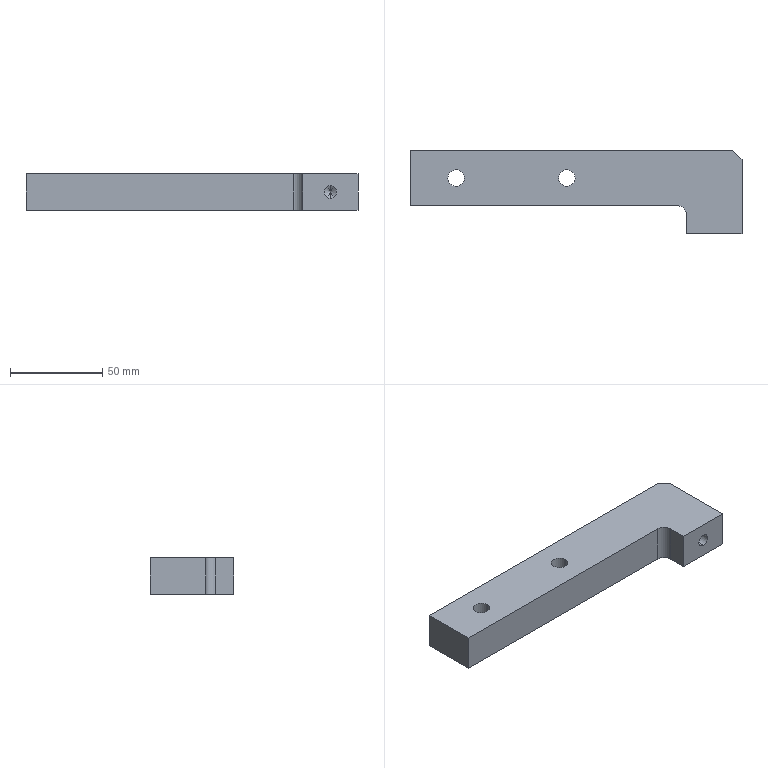Part | SolidWorks | features HoleWzd 2, Chamfer 1, Extrusion 1, Fillet 1, ICE 1 | 1 solid | 24 faces | box 180 x 45 x 20 mm | volume 111535 mm3 | cylinder 11 | plane 11 | cone 2 | commonest cylinder face diameters 9 x4 15 x4 6.8 x2 10 x1
STEP:
#1=CARTESIAN_POINT('',(2.5,0.,9.));
#2=VERTEX_POINT('',#1);
#3=CARTESIAN_POINT('',(-12.5,0.,9.));
#4=VERTEX_POINT('',#3);
#5=CARTESIAN_POINT('',(-5.,0.,9.));
#6=DIRECTION('',(0.,0.,-1.));
#7=DIRECTION('',(-1.,0.,0.));
#8=AXIS2_PLACEMENT_3D('',#5,#6,#7);
#9=CIRCLE('',#8,7.5);
#10=EDGE_CURVE('',#2,#4,#9,.T.);
#11=ORIENTED_EDGE('',*,*,#10,.F.);
#12=CARTESIAN_POINT('',(2.5,0.,0.));
#13=VERTEX_POINT('',#12);
#14=CARTESIAN_POINT('',(2.5,0.,0.));
#15=DIRECTION('',(0.,0.,-1.));
#16=VECTOR('',#15,1000.);
#17=LINE('',#14,#16);
#18=EDGE_CURVE('',#2,#13,#17,.T.);
#19=ORIENTED_EDGE('',*,*,#18,.T.);
#20=CARTESIAN_POINT('',(-12.5,0.,0.));
#21=VERTEX_POINT('',#20);
#22=CARTESIAN_POINT('',(-5.,0.,0.));
#23=DIRECTION('',(0.,0.,-1.));
#24=DIRECTION('',(-1.,0.,0.));
#25=AXIS2_PLACEMENT_3D('',#22,#23,#24);
#26=CIRCLE('',#25,7.5);
#27=EDGE_CURVE('',#13,#21,#26,.T.);
#28=ORIENTED_EDGE('',*,*,#27,.T.);
#29=CARTESIAN_POINT('',(-12.5,0.,0.));
#30=DIRECTION('',(0.,0.,-1.));
#31=VECTOR('',#30,1000.);
#32=LINE('',#29,#31);
#33=EDGE_CURVE('',#4,#21,#32,.T.);
#34=ORIENTED_EDGE('',*,*,#33,.F.);
#35=EDGE_LOOP('',(#11,#19,#28,#34));
#36=FACE_OUTER_BOUND('',#35,.T.);
#37=CARTESIAN_POINT('',(-5.,0.,0.));
#38=DIRECTION('',(0.,0.,-1.));
#39=DIRECTION('',(-1.,0.,0.));
#40=AXIS2_PLACEMENT_3D('',#37,#38,#39);
#41=CYLINDRICAL_SURFACE('',#40,7.5);
#42=ADVANCED_FACE('',(#36),#41,.F.);
#43=CARTESIAN_POINT('',(-9.5,0.,20.));
#44=VERTEX_POINT('',#43);
#45=CARTESIAN_POINT('',(-0.5,0.,20.));
#46=VERTEX_POINT('',#45);
#47=CARTESIAN_POINT('',(-5.,0.,20.));
#48=DIRECTION('',(0.,0.,1.));
#49=DIRECTION('',(1.,0.,0.));
#50=AXIS2_PLACEMENT_3D('',#47,#48,#49);
#51=CIRCLE('',#50,4.5);
#52=EDGE_CURVE('',#44,#46,#51,.T.);
#53=ORIENTED_EDGE('',*,*,#52,.T.);
#54=CARTESIAN_POINT('',(-0.5,0.,9.));
#55=VERTEX_POINT('',#54);
#56=CARTESIAN_POINT('',(-0.5,0.,0.));
#57=DIRECTION('',(0.,0.,-1.));
#58=VECTOR('',#57,1000.);
#59=LINE('',#56,#58);
#60=EDGE_CURVE('',#46,#55,#59,.T.);
#61=ORIENTED_EDGE('',*,*,#60,.T.);
#62=CARTESIAN_POINT('',(-9.5,0.,9.));
#63=VERTEX_POINT('',#62);
#64=CARTESIAN_POINT('',(-5.,0.,9.));
#65=DIRECTION('',(0.,0.,-1.));
#66=DIRECTION('',(-1.,0.,0.));
#67=AXIS2_PLACEMENT_3D('',#64,#65,#66);
#68=CIRCLE('',#67,4.5);
#69=EDGE_CURVE('',#55,#63,#68,.T.);
#70=ORIENTED_EDGE('',*,*,#69,.T.);
#71=CARTESIAN_POINT('',(-9.5,0.,0.));
#72=DIRECTION('',(0.,0.,-1.));
#73=VECTOR('',#72,1000.);
#74=LINE('',#71,#73);
#75=EDGE_CURVE('',#44,#63,#74,.T.);
#76=ORIENTED_EDGE('',*,*,#75,.F.);
#77=EDGE_LOOP('',(#53,#61,#70,#76));
#78=FACE_OUTER_BOUND('',#77,.T.);
#79=CARTESIAN_POINT('',(-5.,0.,0.));
#80=DIRECTION('',(0.,0.,-1.));
#81=DIRECTION('',(-1.,0.,0.));
#82=AXIS2_PLACEMENT_3D('',#79,#80,#81);
#83=CYLINDRICAL_SURFACE('',#82,4.5);
#84=ADVANCED_FACE('',(#78),#83,.F.);
#85=CARTESIAN_POINT('',(-57.5,0.,9.));
#86=VERTEX_POINT('',#85);
#87=CARTESIAN_POINT('',(-72.5,0.,9.));
#88=VERTEX_POINT('',#87);
#89=CARTESIAN_POINT('',(-65.,0.,9.));
#90=DIRECTION('',(0.,0.,-1.));
#91=DIRECTION('',(-1.,0.,0.));
#92=AXIS2_PLACEMENT_3D('',#89,#90,#91);
#93=CIRCLE('',#92,7.5);
#94=EDGE_CURVE('',#86,#88,#93,.T.);
#95=ORIENTED_EDGE('',*,*,#94,.F.);
#96=CARTESIAN_POINT('',(-57.5,0.,0.));
#97=VERTEX_POINT('',#96);
#98=CARTESIAN_POINT('',(-57.5,0.,0.));
#99=DIRECTION('',(0.,0.,-1.));
#100=VECTOR('',#99,1000.);
#101=LINE('',#98,#100);
#102=EDGE_CURVE('',#86,#97,#101,.T.);
#103=ORIENTED_EDGE('',*,*,#102,.T.);
#104=CARTESIAN_POINT('',(-72.5,0.,0.));
#105=VERTEX_POINT('',#104);
#106=CARTESIAN_POINT('',(-65.,0.,0.));
#107=DIRECTION('',(0.,0.,-1.));
#108=DIRECTION('',(-1.,0.,0.));
#109=AXIS2_PLACEMENT_3D('',#106,#107,#108);
#110=CIRCLE('',#109,7.5);
#111=EDGE_CURVE('',#97,#105,#110,.T.);
#112=ORIENTED_EDGE('',*,*,#111,.T.);
#113=CARTESIAN_POINT('',(-72.5,0.,0.));
#114=DIRECTION('',(0.,0.,-1.));
#115=VECTOR('',#114,1000.);
#116=LINE('',#113,#115);
#117=EDGE_CURVE('',#88,#105,#116,.T.);
#118=ORIENTED_EDGE('',*,*,#117,.F.);
#119=EDGE_LOOP('',(#95,#103,#112,#118));
#120=FACE_OUTER_BOUND('',#119,.T.);
#121=CARTESIAN_POINT('',(-65.,0.,0.));
#122=DIRECTION('',(0.,0.,-1.));
#123=DIRECTION('',(-1.,0.,0.));
#124=AXIS2_PLACEMENT_3D('',#121,#122,#123);
#125=CYLINDRICAL_SURFACE('',#124,7.5);
#126=ADVANCED_FACE('',(#120),#125,.F.);
#127=CARTESIAN_POINT('',(-69.5,0.,20.));
#128=VERTEX_POINT('',#127);
#129=CARTESIAN_POINT('',(-60.5,0.,20.));
#130=VERTEX_POINT('',#129);
#131=CARTESIAN_POINT('',(-65.,0.,20.));
#132=DIRECTION('',(0.,0.,1.));
#133=DIRECTION('',(1.,0.,0.));
#134=AXIS2_PLACEMENT_3D('',#131,#132,#133);
#135=CIRCLE('',#134,4.5);
#136=EDGE_CURVE('',#128,#130,#135,.T.);
#137=ORIENTED_EDGE('',*,*,#136,.T.);
#138=CARTESIAN_POINT('',(-60.5,0.,9.));
#139=VERTEX_POINT('',#138);
#140=CARTESIAN_POINT('',(-60.5,0.,0.));
#141=DIRECTION('',(0.,0.,-1.));
#142=VECTOR('',#141,1000.);
#143=LINE('',#140,#142);
#144=EDGE_CURVE('',#130,#139,#143,.T.);
#145=ORIENTED_EDGE('',*,*,#144,.T.);
#146=CARTESIAN_POINT('',(-69.5,0.,9.));
#147=VERTEX_POINT('',#146);
#148=CARTESIAN_POINT('',(-65.,0.,9.));
#149=DIRECTION('',(0.,0.,-1.));
#150=DIRECTION('',(-1.,0.,0.));
#151=AXIS2_PLACEMENT_3D('',#148,#149,#150);
#152=CIRCLE('',#151,4.5);
#153=EDGE_CURVE('',#139,#147,#152,.T.);
#154=ORIENTED_EDGE('',*,*,#153,.T.);
#155=CARTESIAN_POINT('',(-69.5,0.,0.));
#156=DIRECTION('',(0.,0.,-1.));
#157=VECTOR('',#156,1000.);
#158=LINE('',#155,#157);
#159=EDGE_CURVE('',#128,#147,#158,.T.);
#160=ORIENTED_EDGE('',*,*,#159,.F.);
#161=EDGE_LOOP('',(#137,#145,#154,#160));
#162=FACE_OUTER_BOUND('',#161,.T.);
#163=CARTESIAN_POINT('',(-65.,0.,0.));
#164=DIRECTION('',(0.,0.,-1.));
#165=DIRECTION('',(-1.,0.,0.));
#166=AXIS2_PLACEMENT_3D('',#163,#164,#165);
#167=CYLINDRICAL_SURFACE('',#166,4.5);
#168=ADVANCED_FACE('',(#162),#167,.F.);
#169=CARTESIAN_POINT('',(75.,-10.25,13.4));
#170=VERTEX_POINT('',#169);
#171=CARTESIAN_POINT('',(75.,-10.25,6.6));
#172=VERTEX_POINT('',#171);
#173=CARTESIAN_POINT('',(75.,-10.25,10.));
#174=DIRECTION('',(0.,-1.,0.));
#175=DIRECTION('',(0.,0.,-1.));
#176=AXIS2_PLACEMENT_3D('',#173,#174,#175);
#177=CIRCLE('',#176,3.4);
#178=EDGE_CURVE('',#170,#172,#177,.T.);
#179=ORIENTED_EDGE('',*,*,#178,.F.);
#180=CARTESIAN_POINT('',(75.,-30.,13.4));
#181=VERTEX_POINT('',#180);
#182=CARTESIAN_POINT('',(75.,-30.,13.4));
#183=DIRECTION('',(0.,-1.,0.));
#184=VECTOR('',#183,1000.);
#185=LINE('',#182,#184);
#186=EDGE_CURVE('',#170,#181,#185,.T.);
#187=ORIENTED_EDGE('',*,*,#186,.T.);
#188=CARTESIAN_POINT('',(75.,-30.,6.6));
#189=VERTEX_POINT('',#188);
#190=CARTESIAN_POINT('',(75.,-30.,10.));
#191=DIRECTION('',(0.,-1.,0.));
#192=DIRECTION('',(0.,0.,-1.));
#193=AXIS2_PLACEMENT_3D('',#190,#191,#192);
#194=CIRCLE('',#193,3.4);
#195=EDGE_CURVE('',#181,#189,#194,.T.);
#196=ORIENTED_EDGE('',*,*,#195,.T.);
#197=CARTESIAN_POINT('',(75.,-30.,6.6));
#198=DIRECTION('',(0.,-1.,0.));
#199=VECTOR('',#198,1000.);
#200=LINE('',#197,#199);
#201=EDGE_CURVE('',#172,#189,#200,.T.);
#202=ORIENTED_EDGE('',*,*,#201,.F.);
#203=EDGE_LOOP('',(#179,#187,#196,#202));
#204=FACE_OUTER_BOUND('',#203,.T.);
#205=CARTESIAN_POINT('',(75.,-30.,10.));
#206=DIRECTION('',(0.,-1.,0.));
#207=DIRECTION('',(0.,0.,-1.));
#208=AXIS2_PLACEMENT_3D('',#205,#206,#207);
#209=CYLINDRICAL_SURFACE('',#208,3.4);
#210=ADVANCED_FACE('',(#204),#209,.F.);
#211=CARTESIAN_POINT('',(75.,-8.207,10.));
#212=VERTEX_POINT('',#211);
#213=CARTESIAN_POINT('',(75.,-10.25,6.6));
#214=DIRECTION('',(0.,-0.515,-0.8572));
#215=VECTOR('',#214,1000.);
#216=LINE('',#213,#215);
#217=EDGE_CURVE('',#212,#172,#216,.T.);
#218=ORIENTED_EDGE('',*,*,#217,.F.);
#219=CARTESIAN_POINT('',(75.,-10.25,13.4));
#220=DIRECTION('',(0.,-0.515,0.8572));
#221=VECTOR('',#220,1000.);
#222=LINE('',#219,#221);
#223=EDGE_CURVE('',#212,#170,#222,.T.);
#224=ORIENTED_EDGE('',*,*,#223,.T.);
#225=ORIENTED_EDGE('',*,*,#178,.T.);
#226=EDGE_LOOP('',(#218,#224,#225));
#227=FACE_OUTER_BOUND('',#226,.T.);
#228=CARTESIAN_POINT('',(75.,-10.25,10.));
#229=DIRECTION('',(0.,-1.,0.));
#230=DIRECTION('',(0.,0.,-1.));
#231=AXIS2_PLACEMENT_3D('',#228,#229,#230);
#232=CONICAL_SURFACE('',#231,3.4,1.03);
#233=ADVANCED_FACE('',(#227),#232,.F.);
#234=CARTESIAN_POINT('',(90.,-30.,0.));
#235=VERTEX_POINT('',#234);
#236=CARTESIAN_POINT('',(90.,10.,0.));
#237=VERTEX_POINT('',#236);
#238=CARTESIAN_POINT('',(90.,15.,0.));
#239=DIRECTION('',(0.,1.,0.));
#240=VECTOR('',#239,1000.);
#241=LINE('',#238,#240);
#242=EDGE_CURVE('',#235,#237,#241,.T.);
#243=ORIENTED_EDGE('',*,*,#242,.T.);
#244=CARTESIAN_POINT('',(90.,10.,20.));
#245=VERTEX_POINT('',#244);
#246=CARTESIAN_POINT('',(90.,10.,20.));
#247=DIRECTION('',(0.,0.,1.));
#248=VECTOR('',#247,1000.);
#249=LINE('',#246,#248);
#250=EDGE_CURVE('',#237,#245,#249,.T.);
#251=ORIENTED_EDGE('',*,*,#250,.T.);
#252=CARTESIAN_POINT('',(90.,-30.,20.));
#253=VERTEX_POINT('',#252);
#254=CARTESIAN_POINT('',(90.,15.,20.));
#255=DIRECTION('',(0.,1.,0.));
#256=VECTOR('',#255,1000.);
#257=LINE('',#254,#256);
#258=EDGE_CURVE('',#253,#245,#257,.T.);
#259=ORIENTED_EDGE('',*,*,#258,.F.);
#260=CARTESIAN_POINT('',(90.,-30.,-33.541));
#261=DIRECTION('',(0.,0.,1.));
#262=VECTOR('',#261,1000.);
#263=LINE('',#260,#262);
#264=EDGE_CURVE('',#235,#253,#263,.T.);
#265=ORIENTED_EDGE('',*,*,#264,.F.);
#266=EDGE_LOOP('',(#243,#251,#259,#265));
#267=FACE_OUTER_BOUND('',#266,.T.);
#268=CARTESIAN_POINT('',(90.,15.,20.));
#269=DIRECTION('',(-1.,0.,0.));
#270=DIRECTION('',(0.,0.,1.));
#271=AXIS2_PLACEMENT_3D('',#268,#269,#270);
#272=PLANE('',#271);
#273=ADVANCED_FACE('',(#267),#272,.F.);
#274=CARTESIAN_POINT('',(85.,15.,20.));
#275=VERTEX_POINT('',#274);
#276=CARTESIAN_POINT('',(-90.,15.,20.));
#277=VERTEX_POINT('',#276);
#278=CARTESIAN_POINT('',(-90.,15.,20.));
#279=DIRECTION('',(-1.,0.,0.));
#280=VECTOR('',#279,1000.);
#281=LINE('',#278,#280);
#282=EDGE_CURVE('',#275,#277,#281,.T.);
#283=ORIENTED_EDGE('',*,*,#282,.F.);
#284=CARTESIAN_POINT('',(85.,15.,0.));
#285=VERTEX_POINT('',#284);
#286=CARTESIAN_POINT('',(85.,15.,20.));
#287=DIRECTION('',(0.,0.,-1.));
#288=VECTOR('',#287,1000.);
#289=LINE('',#286,#288);
#290=EDGE_CURVE('',#275,#285,#289,.T.);
#291=ORIENTED_EDGE('',*,*,#290,.T.);
#292=CARTESIAN_POINT('',(-90.,15.,0.));
#293=VERTEX_POINT('',#292);
#294=CARTESIAN_POINT('',(-90.,15.,0.));
#295=DIRECTION('',(-1.,0.,0.));
#296=VECTOR('',#295,1000.);
#297=LINE('',#294,#296);
#298=EDGE_CURVE('',#285,#293,#297,.T.);
#299=ORIENTED_EDGE('',*,*,#298,.T.);
#300=CARTESIAN_POINT('',(-90.,15.,20.));
#301=DIRECTION('',(0.,0.,-1.));
#302=VECTOR('',#301,1000.);
#303=LINE('',#300,#302);
#304=EDGE_CURVE('',#277,#293,#303,.T.);
#305=ORIENTED_EDGE('',*,*,#304,.F.);
#306=EDGE_LOOP('',(#283,#291,#299,#305));
#307=FACE_OUTER_BOUND('',#306,.T.);
#308=CARTESIAN_POINT('',(-90.,15.,20.));
#309=DIRECTION('',(0.,-1.,0.));
#310=DIRECTION('',(0.,0.,-1.));
#311=AXIS2_PLACEMENT_3D('',#308,#309,#310);
#312=PLANE('',#311);
#313=ADVANCED_FACE('',(#307),#312,.F.);
#314=CARTESIAN_POINT('',(-90.,-15.,0.));
#315=VERTEX_POINT('',#314);
#316=CARTESIAN_POINT('',(-90.,15.,0.));
#317=DIRECTION('',(0.,-1.,0.));
#318=VECTOR('',#317,1000.);
#319=LINE('',#316,#318);
#320=EDGE_CURVE('',#293,#315,#319,.T.);
#321=ORIENTED_EDGE('',*,*,#320,.T.);
#322=CARTESIAN_POINT('',(-90.,-15.,20.));
#323=VERTEX_POINT('',#322);
#324=CARTESIAN_POINT('',(-90.,-15.,20.));
#325=DIRECTION('',(0.,0.,-1.));
#326=VECTOR('',#325,1000.);
#327=LINE('',#324,#326);
#328=EDGE_CURVE('',#323,#315,#327,.T.);
#329=ORIENTED_EDGE('',*,*,#328,.F.);
#330=CARTESIAN_POINT('',(-90.,15.,20.));
#331=DIRECTION('',(0.,-1.,0.));
#332=VECTOR('',#331,1000.);
#333=LINE('',#330,#332);
#334=EDGE_CURVE('',#277,#323,#333,.T.);
#335=ORIENTED_EDGE('',*,*,#334,.F.);
#336=ORIENTED_EDGE('',*,*,#304,.T.);
#337=EDGE_LOOP('',(#321,#329,#335,#336));
#338=FACE_OUTER_BOUND('',#337,.T.);
#339=CARTESIAN_POINT('',(-90.,15.,20.));
#340=DIRECTION('',(1.,0.,0.));
#341=DIRECTION('',(0.,0.,-1.));
#342=AXIS2_PLACEMENT_3D('',#339,#340,#341);
#343=PLANE('',#342);
#344=ADVANCED_FACE('',(#338),#343,.F.);
#345=CARTESIAN_POINT('',(55.,-15.,0.));
#346=VERTEX_POINT('',#345);
#347=CARTESIAN_POINT('',(-90.,-15.,0.));
#348=DIRECTION('',(1.,0.,0.));
#349=VECTOR('',#348,1000.);
#350=LINE('',#347,#349);
#351=EDGE_CURVE('',#315,#346,#350,.T.);
#352=ORIENTED_EDGE('',*,*,#351,.T.);
#353=CARTESIAN_POINT('',(55.,-15.,20.));
#354=VERTEX_POINT('',#353);
#355=CARTESIAN_POINT('',(55.,-15.,20.));
#356=DIRECTION('',(0.,0.,1.));
#357=VECTOR('',#356,1000.);
#358=LINE('',#355,#357);
#359=EDGE_CURVE('',#346,#354,#358,.T.);
#360=ORIENTED_EDGE('',*,*,#359,.T.);
#361=CARTESIAN_POINT('',(-90.,-15.,20.));
#362=DIRECTION('',(1.,0.,0.));
#363=VECTOR('',#362,1000.);
#364=LINE('',#361,#363);
#365=EDGE_CURVE('',#323,#354,#364,.T.);
#366=ORIENTED_EDGE('',*,*,#365,.F.);
#367=ORIENTED_EDGE('',*,*,#328,.T.);
#368=EDGE_LOOP('',(#352,#360,#366,#367));
#369=FACE_OUTER_BOUND('',#368,.T.);
#370=CARTESIAN_POINT('',(-90.,-15.,20.));
#371=DIRECTION('',(0.,1.,0.));
#372=DIRECTION('',(0.,0.,1.));
#373=AXIS2_PLACEMENT_3D('',#370,#371,#372);
#374=PLANE('',#373);
#375=ADVANCED_FACE('',(#369),#374,.F.);
#376=ORIENTED_EDGE('',*,*,#52,.F.);
#377=CARTESIAN_POINT('',(-5.,0.,20.));
#378=DIRECTION('',(0.,0.,1.));
#379=DIRECTION('',(1.,0.,0.));
#380=AXIS2_PLACEMENT_3D('',#377,#378,#379);
#381=CIRCLE('',#380,4.5);
#382=EDGE_CURVE('',#46,#44,#381,.T.);
#383=ORIENTED_EDGE('',*,*,#382,.F.);
#384=EDGE_LOOP('',(#376,#383));
#385=FACE_BOUND('',#384,.T.);
#386=ORIENTED_EDGE('',*,*,#136,.F.);
#387=CARTESIAN_POINT('',(-65.,0.,20.));
#388=DIRECTION('',(0.,0.,1.));
#389=DIRECTION('',(1.,0.,0.));
#390=AXIS2_PLACEMENT_3D('',#387,#388,#389);
#391=CIRCLE('',#390,4.5);
#392=EDGE_CURVE('',#130,#128,#391,.T.);
#393=ORIENTED_EDGE('',*,*,#392,.F.);
#394=EDGE_LOOP('',(#386,#393));
#395=FACE_BOUND('',#394,.T.);
#396=ORIENTED_EDGE('',*,*,#258,.T.);
#397=CARTESIAN_POINT('',(50.,50.,20.));
#398=DIRECTION('',(-0.7071,0.7071,0.));
#399=VECTOR('',#398,1000.);
#400=LINE('',#397,#399);
#401=EDGE_CURVE('',#245,#275,#400,.T.);
#402=ORIENTED_EDGE('',*,*,#401,.T.);
#403=ORIENTED_EDGE('',*,*,#282,.T.);
#404=ORIENTED_EDGE('',*,*,#334,.T.);
#405=ORIENTED_EDGE('',*,*,#365,.T.);
#406=CARTESIAN_POINT('',(60.,-20.,20.));
#407=VERTEX_POINT('',#406);
#408=CARTESIAN_POINT('',(55.,-20.,20.));
#409=DIRECTION('',(0.,0.,-1.));
#410=DIRECTION('',(1.,0.,0.));
#411=AXIS2_PLACEMENT_3D('',#408,#409,#410);
#412=CIRCLE('',#411,5.);
#413=EDGE_CURVE('',#354,#407,#412,.T.);
#414=ORIENTED_EDGE('',*,*,#413,.T.);
#415=CARTESIAN_POINT('',(60.,-30.,20.));
#416=VERTEX_POINT('',#415);
#417=CARTESIAN_POINT('',(60.,-30.,20.));
#418=DIRECTION('',(0.,1.,0.));
#419=VECTOR('',#418,1000.);
#420=LINE('',#417,#419);
#421=EDGE_CURVE('',#416,#407,#420,.T.);
#422=ORIENTED_EDGE('',*,*,#421,.F.);
#423=CARTESIAN_POINT('',(90.,-30.,20.));
#424=DIRECTION('',(-1.,0.,0.));
#425=VECTOR('',#424,1000.);
#426=LINE('',#423,#425);
#427=EDGE_CURVE('',#253,#416,#426,.T.);
#428=ORIENTED_EDGE('',*,*,#427,.F.);
#429=EDGE_LOOP('',(#396,#402,#403,#404,#405,#414,#422,#428));
#430=FACE_OUTER_BOUND('',#429,.T.);
#431=CARTESIAN_POINT('',(0.,0.,20.));
#432=DIRECTION('',(0.,0.,1.));
#433=DIRECTION('',(1.,0.,0.));
#434=AXIS2_PLACEMENT_3D('',#431,#432,#433);
#435=PLANE('',#434);
#436=ADVANCED_FACE('',(#385,#395,#430),#435,.T.);
#437=CARTESIAN_POINT('',(-5.,0.,0.));
#438=DIRECTION('',(0.,0.,-1.));
#439=DIRECTION('',(-1.,0.,0.));
#440=AXIS2_PLACEMENT_3D('',#437,#438,#439);
#441=CIRCLE('',#440,7.5);
#442=EDGE_CURVE('',#21,#13,#441,.T.);
#443=ORIENTED_EDGE('',*,*,#442,.F.);
#444=ORIENTED_EDGE('',*,*,#27,.F.);
#445=EDGE_LOOP('',(#443,#444));
#446=FACE_BOUND('',#445,.T.);
#447=CARTESIAN_POINT('',(-65.,0.,0.));
#448=DIRECTION('',(0.,0.,-1.));
#449=DIRECTION('',(-1.,0.,0.));
#450=AXIS2_PLACEMENT_3D('',#447,#448,#449);
#451=CIRCLE('',#450,7.5);
#452=EDGE_CURVE('',#105,#97,#451,.T.);
#453=ORIENTED_EDGE('',*,*,#452,.F.);
#454=ORIENTED_EDGE('',*,*,#111,.F.);
#455=EDGE_LOOP('',(#453,#454));
#456=FACE_BOUND('',#455,.T.);
#457=ORIENTED_EDGE('',*,*,#298,.F.);
#458=CARTESIAN_POINT('',(85.,15.,0.));
#459=DIRECTION('',(0.7071,-0.7071,0.));
#460=VECTOR('',#459,1000.);
#461=LINE('',#458,#460);
#462=EDGE_CURVE('',#285,#237,#461,.T.);
#463=ORIENTED_EDGE('',*,*,#462,.T.);
#464=ORIENTED_EDGE('',*,*,#242,.F.);
#465=CARTESIAN_POINT('',(60.,-30.,0.));
#466=VERTEX_POINT('',#465);
#467=CARTESIAN_POINT('',(90.,-30.,0.));
#468=DIRECTION('',(1.,0.,0.));
#469=VECTOR('',#468,1000.);
#470=LINE('',#467,#469);
#471=EDGE_CURVE('',#466,#235,#470,.T.);
#472=ORIENTED_EDGE('',*,*,#471,.F.);
#473=CARTESIAN_POINT('',(60.,-20.,0.));
#474=VERTEX_POINT('',#473);
#475=CARTESIAN_POINT('',(60.,-30.,0.));
#476=DIRECTION('',(0.,-1.,0.));
#477=VECTOR('',#476,1000.);
#478=LINE('',#475,#477);
#479=EDGE_CURVE('',#474,#466,#478,.T.);
#480=ORIENTED_EDGE('',*,*,#479,.F.);
#481=CARTESIAN_POINT('',(55.,-20.,0.));
#482=DIRECTION('',(0.,0.,1.));
#483=DIRECTION('',(1.,0.,0.));
#484=AXIS2_PLACEMENT_3D('',#481,#482,#483);
#485=CIRCLE('',#484,5.);
#486=EDGE_CURVE('',#474,#346,#485,.T.);
#487=ORIENTED_EDGE('',*,*,#486,.T.);
#488=ORIENTED_EDGE('',*,*,#351,.F.);
#489=ORIENTED_EDGE('',*,*,#320,.F.);
#490=EDGE_LOOP('',(#457,#463,#464,#472,#480,#487,#488,#489));
#491=FACE_OUTER_BOUND('',#490,.T.);
#492=CARTESIAN_POINT('',(0.,0.,0.));
#493=DIRECTION('',(0.,0.,1.));
#494=DIRECTION('',(1.,0.,0.));
#495=AXIS2_PLACEMENT_3D('',#492,#493,#494);
#496=PLANE('',#495);
#497=ADVANCED_FACE('',(#446,#456,#491),#496,.F.);
#498=ORIENTED_EDGE('',*,*,#421,.T.);
#499=CARTESIAN_POINT('',(60.,-20.,0.));
#500=DIRECTION('',(0.,0.,-1.));
#501=VECTOR('',#500,1000.);
#502=LINE('',#499,#501);
#503=EDGE_CURVE('',#407,#474,#502,.T.);
#504=ORIENTED_EDGE('',*,*,#503,.T.);
#505=ORIENTED_EDGE('',*,*,#479,.T.);
#506=CARTESIAN_POINT('',(60.,-30.,-33.541));
#507=DIRECTION('',(0.,0.,1.));
#508=VECTOR('',#507,1000.);
#509=LINE('',#506,#508);
#510=EDGE_CURVE('',#466,#416,#509,.T.);
#511=ORIENTED_EDGE('',*,*,#510,.T.);
#512=EDGE_LOOP('',(#498,#504,#505,#511));
#513=FACE_OUTER_BOUND('',#512,.T.);
#514=CARTESIAN_POINT('',(60.,-30.,-33.541));
#515=DIRECTION('',(1.,0.,0.));
#516=DIRECTION('',(0.,0.,-1.));
#517=AXIS2_PLACEMENT_3D('',#514,#515,#516);
#518=PLANE('',#517);
#519=ADVANCED_FACE('',(#513),#518,.F.);
#520=CARTESIAN_POINT('',(75.,-30.,10.));
#521=DIRECTION('',(0.,-1.,0.));
#522=DIRECTION('',(0.,0.,-1.));
#523=AXIS2_PLACEMENT_3D('',#520,#521,#522);
#524=CIRCLE('',#523,3.4);
#525=EDGE_CURVE('',#189,#181,#524,.T.);
#526=ORIENTED_EDGE('',*,*,#525,.F.);
#527=ORIENTED_EDGE('',*,*,#195,.F.);
#528=EDGE_LOOP('',(#526,#527));
#529=FACE_BOUND('',#528,.T.);
#530=ORIENTED_EDGE('',*,*,#510,.F.);
#531=ORIENTED_EDGE('',*,*,#471,.T.);
#532=ORIENTED_EDGE('',*,*,#264,.T.);
#533=ORIENTED_EDGE('',*,*,#427,.T.);
#534=EDGE_LOOP('',(#530,#531,#532,#533));
#535=FACE_OUTER_BOUND('',#534,.T.);
#536=CARTESIAN_POINT('',(90.,-30.,-33.541));
#537=DIRECTION('',(0.,1.,0.));
#538=DIRECTION('',(-1.,0.,0.));
#539=AXIS2_PLACEMENT_3D('',#536,#537,#538);
#540=PLANE('',#539);
#541=ADVANCED_FACE('',(#529,#535),#540,.F.);
#542=ORIENTED_EDGE('',*,*,#486,.F.);
#543=ORIENTED_EDGE('',*,*,#503,.F.);
#544=ORIENTED_EDGE('',*,*,#413,.F.);
#545=ORIENTED_EDGE('',*,*,#359,.F.);
#546=EDGE_LOOP('',(#542,#543,#544,#545));
#547=FACE_OUTER_BOUND('',#546,.T.);
#548=CARTESIAN_POINT('',(55.,-20.,20.));
#549=DIRECTION('',(0.,0.,-1.));
#550=DIRECTION('',(-1.,0.,0.));
#551=AXIS2_PLACEMENT_3D('',#548,#549,#550);
#552=CYLINDRICAL_SURFACE('',#551,5.);
#553=ADVANCED_FACE('',(#547),#552,.F.);
#554=ORIENTED_EDGE('',*,*,#401,.F.);
#555=ORIENTED_EDGE('',*,*,#250,.F.);
#556=ORIENTED_EDGE('',*,*,#462,.F.);
#557=ORIENTED_EDGE('',*,*,#290,.F.);
#558=EDGE_LOOP('',(#554,#555,#556,#557));
#559=FACE_OUTER_BOUND('',#558,.T.);
#560=CARTESIAN_POINT('',(85.,15.,20.));
#561=DIRECTION('',(-0.7071,-0.7071,0.));
#562=DIRECTION('',(0.,0.,-1.));
#563=AXIS2_PLACEMENT_3D('',#560,#561,#562);
#564=PLANE('',#563);
#565=ADVANCED_FACE('',(#559),#564,.F.);
#566=ORIENTED_EDGE('',*,*,#223,.F.);
#567=ORIENTED_EDGE('',*,*,#217,.T.);
#568=CARTESIAN_POINT('',(75.,-10.25,10.));
#569=DIRECTION('',(0.,-1.,0.));
#570=DIRECTION('',(0.,0.,-1.));
#571=AXIS2_PLACEMENT_3D('',#568,#569,#570);
#572=CIRCLE('',#571,3.4);
#573=EDGE_CURVE('',#172,#170,#572,.T.);
#574=ORIENTED_EDGE('',*,*,#573,.T.);
#575=EDGE_LOOP('',(#566,#567,#574));
#576=FACE_OUTER_BOUND('',#575,.T.);
#577=CARTESIAN_POINT('',(75.,-10.25,10.));
#578=DIRECTION('',(0.,-1.,0.));
#579=DIRECTION('',(0.,0.,-1.));
#580=AXIS2_PLACEMENT_3D('',#577,#578,#579);
#581=CONICAL_SURFACE('',#580,3.4,1.03);
#582=ADVANCED_FACE('',(#576),#581,.F.);
#583=ORIENTED_EDGE('',*,*,#186,.F.);
#584=ORIENTED_EDGE('',*,*,#573,.F.);
#585=ORIENTED_EDGE('',*,*,#201,.T.);
#586=ORIENTED_EDGE('',*,*,#525,.T.);
#587=EDGE_LOOP('',(#583,#584,#585,#586));
#588=FACE_OUTER_BOUND('',#587,.T.);
#589=CARTESIAN_POINT('',(75.,-30.,10.));
#590=DIRECTION('',(0.,-1.,0.));
#591=DIRECTION('',(0.,0.,-1.));
#592=AXIS2_PLACEMENT_3D('',#589,#590,#591);
#593=CYLINDRICAL_SURFACE('',#592,3.4);
#594=ADVANCED_FACE('',(#588),#593,.F.);
#595=ORIENTED_EDGE('',*,*,#144,.F.);
#596=ORIENTED_EDGE('',*,*,#392,.T.);
#597=ORIENTED_EDGE('',*,*,#159,.T.);
#598=CARTESIAN_POINT('',(-65.,0.,9.));
#599=DIRECTION('',(0.,0.,-1.));
#600=DIRECTION('',(-1.,0.,0.));
#601=AXIS2_PLACEMENT_3D('',#598,#599,#600);
#602=CIRCLE('',#601,4.5);
#603=EDGE_CURVE('',#147,#139,#602,.T.);
#604=ORIENTED_EDGE('',*,*,#603,.T.);
#605=EDGE_LOOP('',(#595,#596,#597,#604));
#606=FACE_OUTER_BOUND('',#605,.T.);
#607=CARTESIAN_POINT('',(-65.,0.,0.));
#608=DIRECTION('',(0.,0.,-1.));
#609=DIRECTION('',(-1.,0.,0.));
#610=AXIS2_PLACEMENT_3D('',#607,#608,#609);
#611=CYLINDRICAL_SURFACE('',#610,4.5);
#612=ADVANCED_FACE('',(#606),#611,.F.);
#613=ORIENTED_EDGE('',*,*,#603,.F.);
#614=ORIENTED_EDGE('',*,*,#153,.F.);
#615=EDGE_LOOP('',(#613,#614));
#616=FACE_BOUND('',#615,.T.);
#617=CARTESIAN_POINT('',(-65.,0.,9.));
#618=DIRECTION('',(0.,0.,-1.));
#619=DIRECTION('',(-1.,0.,0.));
#620=AXIS2_PLACEMENT_3D('',#617,#618,#619);
#621=CIRCLE('',#620,7.5);
#622=EDGE_CURVE('',#88,#86,#621,.T.);
#623=ORIENTED_EDGE('',*,*,#622,.T.);
#624=ORIENTED_EDGE('',*,*,#94,.T.);
#625=EDGE_LOOP('',(#623,#624));
#626=FACE_OUTER_BOUND('',#625,.T.);
#627=CARTESIAN_POINT('',(-60.5,0.,9.));
#628=DIRECTION('',(0.,0.,1.));
#629=DIRECTION('',(1.,0.,0.));
#630=AXIS2_PLACEMENT_3D('',#627,#628,#629);
#631=PLANE('',#630);
#632=ADVANCED_FACE('',(#616,#626),#631,.F.);
#633=ORIENTED_EDGE('',*,*,#102,.F.);
#634=ORIENTED_EDGE('',*,*,#622,.F.);
#635=ORIENTED_EDGE('',*,*,#117,.T.);
#636=ORIENTED_EDGE('',*,*,#452,.T.);
#637=EDGE_LOOP('',(#633,#634,#635,#636));
#638=FACE_OUTER_BOUND('',#637,.T.);
#639=CARTESIAN_POINT('',(-65.,0.,0.));
#640=DIRECTION('',(0.,0.,-1.));
#641=DIRECTION('',(-1.,0.,0.));
#642=AXIS2_PLACEMENT_3D('',#639,#640,#641);
#643=CYLINDRICAL_SURFACE('',#642,7.5);
#644=ADVANCED_FACE('',(#638),#643,.F.);
#645=ORIENTED_EDGE('',*,*,#60,.F.);
#646=ORIENTED_EDGE('',*,*,#382,.T.);
#647=ORIENTED_EDGE('',*,*,#75,.T.);
#648=CARTESIAN_POINT('',(-5.,0.,9.));
#649=DIRECTION('',(0.,0.,-1.));
#650=DIRECTION('',(-1.,0.,0.));
#651=AXIS2_PLACEMENT_3D('',#648,#649,#650);
#652=CIRCLE('',#651,4.5);
#653=EDGE_CURVE('',#63,#55,#652,.T.);
#654=ORIENTED_EDGE('',*,*,#653,.T.);
#655=EDGE_LOOP('',(#645,#646,#647,#654));
#656=FACE_OUTER_BOUND('',#655,.T.);
#657=CARTESIAN_POINT('',(-5.,0.,0.));
#658=DIRECTION('',(0.,0.,-1.));
#659=DIRECTION('',(-1.,0.,0.));
#660=AXIS2_PLACEMENT_3D('',#657,#658,#659);
#661=CYLINDRICAL_SURFACE('',#660,4.5);
#662=ADVANCED_FACE('',(#656),#661,.F.);
#663=ORIENTED_EDGE('',*,*,#653,.F.);
#664=ORIENTED_EDGE('',*,*,#69,.F.);
#665=EDGE_LOOP('',(#663,#664));
#666=FACE_BOUND('',#665,.T.);
#667=CARTESIAN_POINT('',(-5.,0.,9.));
#668=DIRECTION('',(0.,0.,-1.));
#669=DIRECTION('',(-1.,0.,0.));
#670=AXIS2_PLACEMENT_3D('',#667,#668,#669);
#671=CIRCLE('',#670,7.5);
#672=EDGE_CURVE('',#4,#2,#671,.T.);
#673=ORIENTED_EDGE('',*,*,#672,.T.);
#674=ORIENTED_EDGE('',*,*,#10,.T.);
#675=EDGE_LOOP('',(#673,#674));
#676=FACE_OUTER_BOUND('',#675,.T.);
#677=CARTESIAN_POINT('',(-0.5,0.,9.));
#678=DIRECTION('',(0.,0.,1.));
#679=DIRECTION('',(1.,0.,0.));
#680=AXIS2_PLACEMENT_3D('',#677,#678,#679);
#681=PLANE('',#680);
#682=ADVANCED_FACE('',(#666,#676),#681,.F.);
#683=ORIENTED_EDGE('',*,*,#18,.F.);
#684=ORIENTED_EDGE('',*,*,#672,.F.);
#685=ORIENTED_EDGE('',*,*,#33,.T.);
#686=ORIENTED_EDGE('',*,*,#442,.T.);
#687=EDGE_LOOP('',(#683,#684,#685,#686));
#688=FACE_OUTER_BOUND('',#687,.T.);
#689=CARTESIAN_POINT('',(-5.,0.,0.));
#690=DIRECTION('',(0.,0.,-1.));
#691=DIRECTION('',(-1.,0.,0.));
#692=AXIS2_PLACEMENT_3D('',#689,#690,#691);
#693=CYLINDRICAL_SURFACE('',#692,7.5);
#694=ADVANCED_FACE('',(#688),#693,.F.);
#695=CLOSED_SHELL('',(#42,#84,#126,#168,#210,#233,#273,#313,#344,#375,#436,#497,#519,#541,#553,#565,#582,#594,#612,#632,#644,#662,#682,#694));
#696=MANIFOLD_SOLID_BREP('',#695);
#697=CARTESIAN_POINT('',(0.,0.,0.));
#698=DIRECTION('',(0.,0.,1.));
#699=DIRECTION('',(1.,0.,0.));
#700=AXIS2_PLACEMENT_3D('',#697,#698,#699);
#701=(LENGTH_UNIT()NAMED_UNIT(*)SI_UNIT(.MILLI.,.METRE.));
#702=UNCERTAINTY_MEASURE_WITH_UNIT(LENGTH_MEASURE(0.00001),#701,'','');
#703=(NAMED_UNIT(*)PLANE_ANGLE_UNIT()SI_UNIT($,.RADIAN.));
#704=(NAMED_UNIT(*)SI_UNIT($,.STERADIAN.)SOLID_ANGLE_UNIT());
#705=(GEOMETRIC_REPRESENTATION_CONTEXT(3)GLOBAL_UNCERTAINTY_ASSIGNED_CONTEXT((#702))GLOBAL_UNIT_ASSIGNED_CONTEXT((#701,#703,#704))REPRESENTATION_CONTEXT('',''));
#706=ADVANCED_BREP_SHAPE_REPRESENTATION('',(#696,#700),#705);